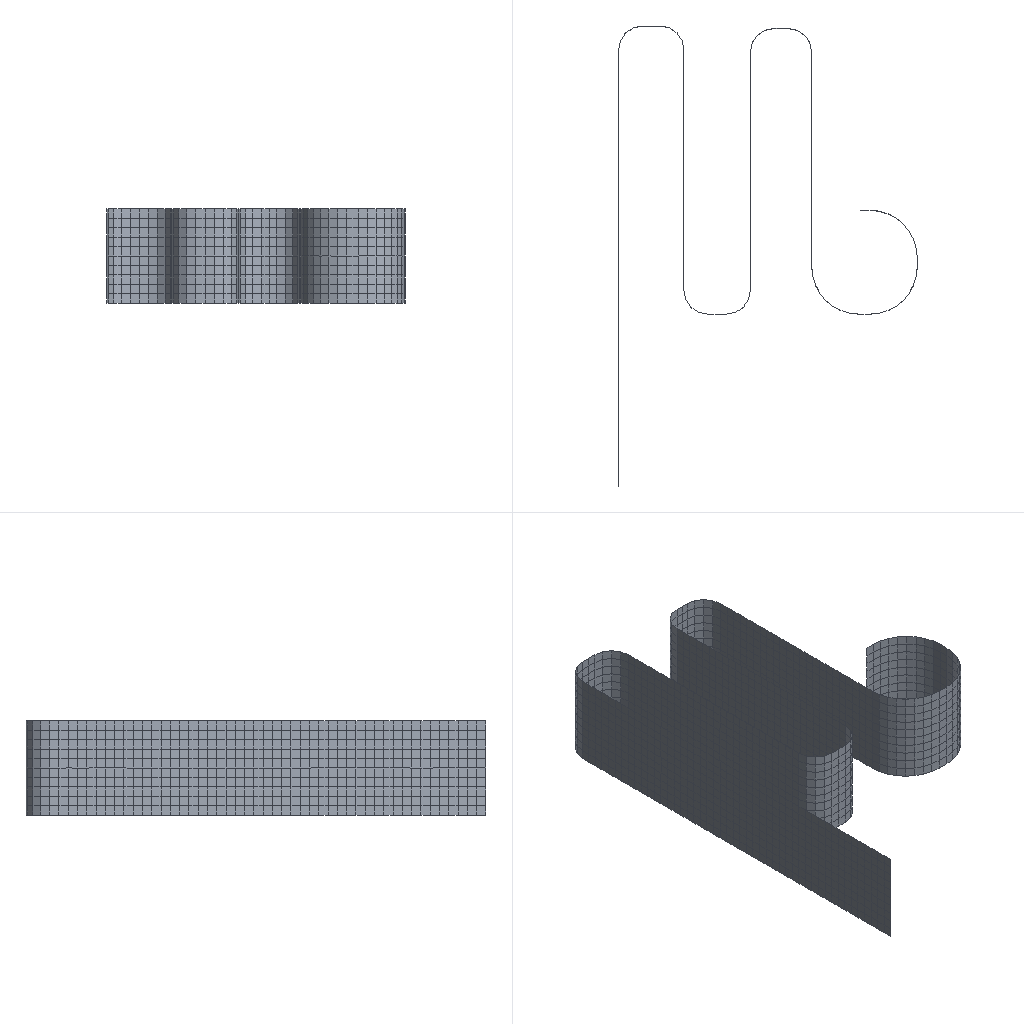Simulation study | ansys workbench
Ansys APDL input file, long lists of numbers shortened:
/batch
/config,noeldb,1     ! force off writing results to database
*get,_wallstrt,active,,time,wall
! ANSYS input file written by Workbench version 2025 R2
! File used for geometry attach:
/title,[REDACTED]
! ****** Begin Custom Load Command Snippet ******
/COM, ACT Extensions:
/COM,     LSDYNA, 2025.2
/COM,/COM,     ANSYSMotion, 2025.2
/COM,
! ****** End   Custom Load Command Snippet ******
*DIM,_wb_ProjectScratch_dir,string,248
_wb_ProjectScratch_dir(1) = ''
*DIM,_wb_SolverFiles_dir,string,248
_wb_SolverFiles_dir(1) = ''
*DIM,_wb_userfiles_dir,string,248
_wb_userfiles_dir(1) = ''
/com,--- Data in consistent NMM units. See Solving Units in the help system for more information.
/units,MPA
/nopr
/wb,file,start              !  signify a WB generated input file
/prep7
! Turn off shape checking because checks already performed inside WB mesher.
! See help system for more information.
SHPP,OFF,,NOWARN
/nolist
etcon,set             ! allow ANSYS to choose best KEYOP's for 180x elements, resets any applicable keyopt to MAPDL defaults
/com,*********** Send User Defined Coordinate System(s) ***********
csys,0
/com,*********** Nodes for the whole assembly ***********
nblock,3,,2178
(1i9,3e20.9e3)
        1     2.046204580E+01     1.679463945E+01     5.000001091E+00
! (1979 more lines like these left out)
-1
/wb,elem,start            !  set before creation of elements
/com,*********** Elements for Body 1 'Surface Body' ***********
et,1,181
keyo,1,1,0          ! bending and membrane stiffness
keyo,1,3,2
MAT,1 $ TYPE,1 $ REAL,1 $ SECNUM,1 $ ESYS,0
eblock,11,COMPACT,,1790
(11i9)
        1        5        7       10       13
! (1789 more lines like these left out)
-1
secnum,1    ! reset the section ID to default
/wb,elem,end               !  done creating elements
toffst,273.15,      ! Temperature offset from absolute zero
/com,*********** Set Reference Temperature ***********
tref,22.
/wb,mat,start              !  starting to send materials
/com,*********** Send Materials ***********
Temperature = 'TEMP' ! Temperature
MP,DENS,1,7.85e-09,	! tonne mm^-3
MP,ALPX,1,1.2e-05,	! C^-1
MP,C,1,434000000,	! mm^2 s^-2 C^-1
MP,KXX,1,60.5,	! tonne mm s^-3 C^-1
MP,RSVX,1,0.00017,	! ohm mm
MP,EX,1,200000,	! tonne s^-2 mm^-1
MP,NUXY,1,0.3,
MP,MURX,1,10000,
/wb,mat,end                !  done sending materials
/com,*********** Send Sheet Properties ***********
sectype,1,shell
secdata,1.
secoff,mid
!************************* Model Summary ********************
!Surface Body,	Structural steel,	matid,	1
!************************* End Model Summary ********************
! get the diagonal of the bounding box. Needed later for other things
*get,_xmin,node,,mnloc,x
*get,_ymin,node,,mnloc,y
*get,_zmin,node,,mnloc,z
*get,_xmax,node,,mxloc,x
*get,_ymax,node,,mxloc,y
*get,_zmax,node,,mxloc,z
_ASMDIAG=(_xmax-_xmin)*(_xmax-_xmin)+(_ymax-_ymin)*(_ymax-_ymin)+(_zmax-_zmin)*(_zmax-_zmin)
_ASMDIAG=SQRT(_ASMDIAG)
/wb,contact,start          !  starting to send contact
/wb,contact,end            !  done creating contacts
/golist
/wb,load,start             !  starting to send loads
/com,*********** Fixed Supports ***********
CMBLOCK,_FIXEDSU,NODE,       11
(8i10)
       113       126       138       149       162       176       188       201
       215      1528      1531
cmsel,s,_FIXEDSU
d,all,all
nsel,all
/com,*********** Define Force Using Surface Effect Elements ***********
local,12,0,0.,0.,0.,0.,0.,0.
csys,0
et,2,156
keyop,2,5,1         !  No orientation node
MAT,2 $ TYPE,2 $ REAL,2 $ SECNUM,2 $ ESYS,12
eblock,11,COMPACT,,10
(11i9)
     1791      195      200
! (9 more lines like these left out)
-1
secnum,1    ! reset the section ID to default
esel,s,type,,2
keyop,2,2,1         ! Apply load in local coordinate system
keyop,2,7,1         ! Use original area so load is constant in large deformation
esel,all
/gst,on,on
fini
*get,_numnode,node,0,count
*get,_numelem,elem,0,count
*get, _MAXELEMNUM, elem, 0, NUM, MAX
*get, _MAXNODENUM, node, 0, NUM, MAX
*get, _MAXELEMTYPE, etyp, 0, NUM, MAX
*get, _MAXREALCONST, rcon, 0, NUM, MAX
/go
/wb,load,end               !  done creating loads
/com,--- Number of total nodes = %_numnode%
/com,--- Number of contact elements = 10
/com,--- Number of spring elements = 0
/com,--- Number of bearing elements = 0
/com,--- Number of solid elements = 1790
/com,--- Number of condensed parts = 0
/com,--- Number of total elements = %_numelem%
*get,_wallbsol,active,,time,wall
/com,****************************************************************************
/com,*************************    SOLUTION       ********************************
/com,****************************************************************************
/solu
antype,0                   ! static analysis
_thickRatio=  0     ! Ratio of thick parts in the model
eqsl,sparse,,,,,1
cntr,print,1               ! print out contact info and also make no initial contact an error
cncheck,dmp		!	Enable program controlled contact splitting for distributed memory parallel run
dmpoption,emat,no             ! Don't combine emat file for DANSYS
dmpoption,esav,no             ! Don't combine esav file for DANSYS
nldiag,cont,iter           ! print out contact info each equilibrium iteration
rescontrol,,none                 ! Do not keep any restart files
/com,****************************************************
/com,******************* SOLVE FOR LS 1 OF 1 ****************
esel,s,type,,2
nsle
sfe,all,1,pres,1,25.
sfe,all,2,pres,1,0.
sfe,all,3,pres,1,0.
nsel,all
esel,all
/nopr
/gopr
nsub,1,1,1
time,1.
outres,erase
outres,all,none
outres,nsol,all,
outres,rsol,all
outres,eangl,all
outres,etmp,all
outres,veng,all
outres,strs,all,
outres,epel,all,
outres,eppl,all,
outres,cont,all,
! *********** WB SOLVE COMMAND ***********
! check interactive state
*get,ANSINTER_,active,,int
*if,ANSINTER_,ne,0,then
/eof
*endif
solve
/com *************** Write FE CONNECTORS *********
CEWRITE,file,ce,,INTE
/com,****************************************************
/com,*************** FINISHED SOLVE FOR LS 1 *************
*get,_wallasol,active,,time,wall
/nopr
*get,_numnode,node,0,count
*get,_numelem,elem,0,count
*get, _MAXELEMNUM, elem, 0, NUM, MAX
*get, _MAXNODENUM, node, 0, NUM, MAX,,,INTERNAL
*get, _MAXELEMTYPE, etyp, 0, NUM, MAX
*get, _MAXREALCONST, rcon, 0, NUM, MAX
*get,_NSOLTHREADS,active,0,ntfs
*get,_NSOLPROCESSES,active,0,npfs
/gopr
/post1
xmlo,ENCODING,ISO-8859-1
xmlo,parm
/xml,parm,xml
fini
/gopr
*get,_walldone,active,,time,wall
_preptime=(_wallbsol-_wallstrt)*3600
_solvtime=(_wallasol-_wallbsol)*3600
_posttime=(_walldone-_wallasol)*3600
_totaltim=(_walldone-_wallstrt)*3600
*get,_dlbratio,active,0,solu,dlbr
*get,_combtime,active,0,solu,comb
*get,_ssmode,active,0,solu,ssmm
*get,_ndofs,active,0,solu,ndof
*get,_sol_end_time,active,0,set,time
*if,_sol_end_time,eq,1.,then
/fclean				!clean distributed files
*endif
/com,--- Total number of nodes = %_numnode%
/com,--- Total number of elements = %_numelem%
/com,--- Element load balance ratio = %_dlbratio%
/com,--- Time to combine distributed files = %_combtime%
/com,--- Sparse memory mode = %_ssmode%
/com,--- Number of DOF = %_ndofs%
/wb,file,end               ! done with WB generated input